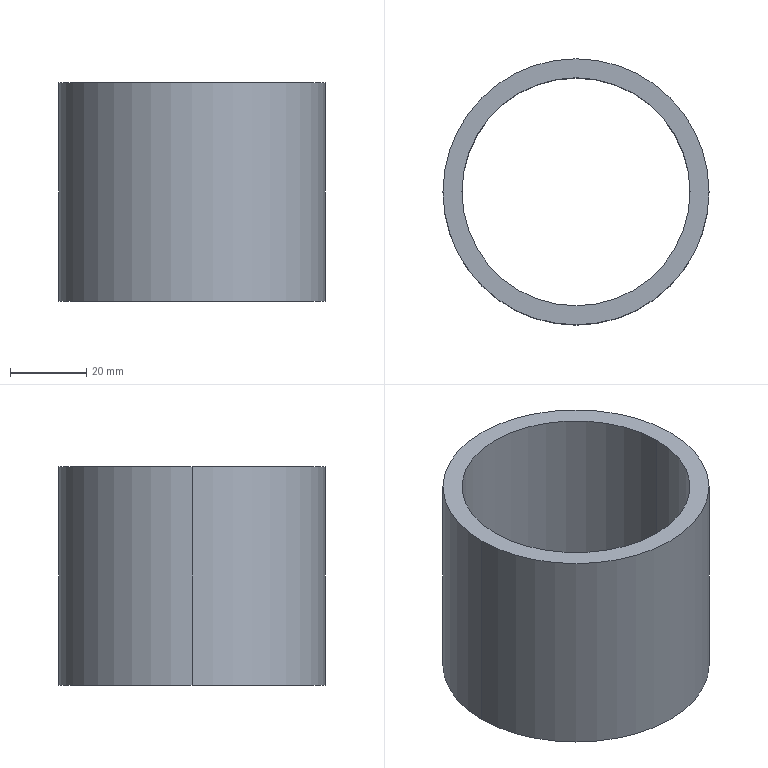Part | STEP file | 05-Spacer 2 | 1 solid | 6 faces | box 70 x 70 x 57.5 mm | volume 58709 mm3 | cylinder 4 | plane 2 | commonest cylinder face diameters 60 x2 70 x2
STEP:
#1=CARTESIAN_POINT('',(0.,0.,0.));
#2=DIRECTION('',(0.,0.,1.));
#3=DIRECTION('',(1.,0.,0.));
#4=AXIS2_PLACEMENT_3D('',#1,#2,#3);
#5=CARTESIAN_POINT('',(-30.,0.,57.5));
#6=VERTEX_POINT('',#5);
#7=CARTESIAN_POINT('',(-30.,0.,0.));
#8=VERTEX_POINT('',#7);
#9=CARTESIAN_POINT('',(-30.,0.,57.5));
#10=DIRECTION('',(0.,0.,-1.));
#11=VECTOR('',#10,1.);
#12=LINE('',#9,#11);
#13=CARTESIAN_POINT('',(0.,0.,57.5));
#14=DIRECTION('',(0.,0.,-1.));
#15=DIRECTION('',(-1.,0.,0.));
#16=AXIS2_PLACEMENT_3D('',#13,#14,#15);
#17=CYLINDRICAL_SURFACE('',#16,30.);
#18=CARTESIAN_POINT('',(6.283,0.));
#19=DIRECTION('',(0.,1.));
#20=VECTOR('',#19,1.);
#21=LINE('',#18,#20);
#22=(GEOMETRIC_REPRESENTATION_CONTEXT(2)PARAMETRIC_REPRESENTATION_CONTEXT()REPRESENTATION_CONTEXT('',''));
#23=DEFINITIONAL_REPRESENTATION('',(#21),#22);
#24=PCURVE('',#17,#23);
#25=CARTESIAN_POINT('',(0.,0.,57.5));
#26=DIRECTION('',(0.,0.,-1.));
#27=DIRECTION('',(-1.,0.,0.));
#28=AXIS2_PLACEMENT_3D('',#25,#26,#27);
#29=CYLINDRICAL_SURFACE('',#28,30.);
#30=CARTESIAN_POINT('',(0.,0.));
#31=DIRECTION('',(0.,1.));
#32=VECTOR('',#31,1.);
#33=LINE('',#30,#32);
#34=(GEOMETRIC_REPRESENTATION_CONTEXT(2)PARAMETRIC_REPRESENTATION_CONTEXT()REPRESENTATION_CONTEXT('',''));
#35=DEFINITIONAL_REPRESENTATION('',(#33),#34);
#36=PCURVE('',#29,#35);
#37=SURFACE_CURVE('',#12,(#24,#36),.PCURVE_S1.);
#38=EDGE_CURVE('',#6,#8,#37,.T.);
#39=ORIENTED_EDGE('',*,*,#38,.T.);
#40=CARTESIAN_POINT('',(30.,0.,0.));
#41=VERTEX_POINT('',#40);
#42=CARTESIAN_POINT('',(0.,0.,0.));
#43=DIRECTION('',(0.,0.,1.));
#44=DIRECTION('',(1.,0.,0.));
#45=AXIS2_PLACEMENT_3D('',#42,#43,#44);
#46=CIRCLE('',#45,30.);
#47=CARTESIAN_POINT('',(9.425,57.5));
#48=DIRECTION('',(-1.,0.));
#49=VECTOR('',#48,1.);
#50=LINE('',#47,#49);
#51=(GEOMETRIC_REPRESENTATION_CONTEXT(2)PARAMETRIC_REPRESENTATION_CONTEXT()REPRESENTATION_CONTEXT('',''));
#52=DEFINITIONAL_REPRESENTATION('',(#50),#51);
#53=PCURVE('',#17,#52);
#54=CARTESIAN_POINT('',(0.,0.,0.));
#55=DIRECTION('',(0.,0.,1.));
#56=DIRECTION('',(1.,0.,0.));
#57=AXIS2_PLACEMENT_3D('',#54,#55,#56);
#58=PLANE('',#57);
#59=CARTESIAN_POINT('',(0.,0.));
#60=DIRECTION('',(1.,0.));
#61=AXIS2_PLACEMENT_2D('',#59,#60);
#62=CIRCLE('',#61,30.);
#63=(GEOMETRIC_REPRESENTATION_CONTEXT(2)PARAMETRIC_REPRESENTATION_CONTEXT()REPRESENTATION_CONTEXT('',''));
#64=DEFINITIONAL_REPRESENTATION('',(#62),#63);
#65=PCURVE('',#58,#64);
#66=SURFACE_CURVE('',#46,(#53,#65),.PCURVE_S1.);
#67=EDGE_CURVE('',#8,#41,#66,.T.);
#68=ORIENTED_EDGE('',*,*,#67,.T.);
#69=CARTESIAN_POINT('',(30.,0.,57.5));
#70=VERTEX_POINT('',#69);
#71=CARTESIAN_POINT('',(30.,0.,57.5));
#72=DIRECTION('',(0.,0.,-1.));
#73=VECTOR('',#72,1.);
#74=LINE('',#71,#73);
#75=CARTESIAN_POINT('',(3.142,0.));
#76=DIRECTION('',(0.,1.));
#77=VECTOR('',#76,1.);
#78=LINE('',#75,#77);
#79=(GEOMETRIC_REPRESENTATION_CONTEXT(2)PARAMETRIC_REPRESENTATION_CONTEXT()REPRESENTATION_CONTEXT('',''));
#80=DEFINITIONAL_REPRESENTATION('',(#78),#79);
#81=PCURVE('',#17,#80);
#82=CARTESIAN_POINT('',(3.142,0.));
#83=DIRECTION('',(0.,1.));
#84=VECTOR('',#83,1.);
#85=LINE('',#82,#84);
#86=(GEOMETRIC_REPRESENTATION_CONTEXT(2)PARAMETRIC_REPRESENTATION_CONTEXT()REPRESENTATION_CONTEXT('',''));
#87=DEFINITIONAL_REPRESENTATION('',(#85),#86);
#88=PCURVE('',#29,#87);
#89=SURFACE_CURVE('',#74,(#81,#88),.PCURVE_S1.);
#90=EDGE_CURVE('',#70,#41,#89,.T.);
#91=ORIENTED_EDGE('',*,*,#90,.F.);
#92=CARTESIAN_POINT('',(0.,0.,57.5));
#93=DIRECTION('',(0.,0.,1.));
#94=DIRECTION('',(1.,0.,0.));
#95=AXIS2_PLACEMENT_3D('',#92,#93,#94);
#96=CIRCLE('',#95,30.);
#97=CARTESIAN_POINT('',(9.425,0.));
#98=DIRECTION('',(-1.,0.));
#99=VECTOR('',#98,1.);
#100=LINE('',#97,#99);
#101=(GEOMETRIC_REPRESENTATION_CONTEXT(2)PARAMETRIC_REPRESENTATION_CONTEXT()REPRESENTATION_CONTEXT('',''));
#102=DEFINITIONAL_REPRESENTATION('',(#100),#101);
#103=PCURVE('',#17,#102);
#104=CARTESIAN_POINT('',(0.,0.,57.5));
#105=DIRECTION('',(0.,0.,1.));
#106=DIRECTION('',(1.,0.,0.));
#107=AXIS2_PLACEMENT_3D('',#104,#105,#106);
#108=PLANE('',#107);
#109=CARTESIAN_POINT('',(0.,0.));
#110=DIRECTION('',(1.,0.));
#111=AXIS2_PLACEMENT_2D('',#109,#110);
#112=CIRCLE('',#111,30.);
#113=(GEOMETRIC_REPRESENTATION_CONTEXT(2)PARAMETRIC_REPRESENTATION_CONTEXT()REPRESENTATION_CONTEXT('',''));
#114=DEFINITIONAL_REPRESENTATION('',(#112),#113);
#115=PCURVE('',#108,#114);
#116=SURFACE_CURVE('',#96,(#103,#115),.PCURVE_S1.);
#117=EDGE_CURVE('',#6,#70,#116,.T.);
#118=ORIENTED_EDGE('',*,*,#117,.F.);
#119=EDGE_LOOP('',(#39,#68,#91,#118));
#120=FACE_BOUND('',#119,.F.);
#121=ADVANCED_FACE('',(#120),#17,.F.);
#122=CARTESIAN_POINT('',(35.,0.,57.5));
#123=VERTEX_POINT('',#122);
#124=CARTESIAN_POINT('',(-35.,0.,57.5));
#125=VERTEX_POINT('',#124);
#126=CARTESIAN_POINT('',(0.,0.,57.5));
#127=DIRECTION('',(0.,0.,1.));
#128=DIRECTION('',(1.,0.,0.));
#129=AXIS2_PLACEMENT_3D('',#126,#127,#128);
#130=CIRCLE('',#129,35.);
#131=CARTESIAN_POINT('',(0.,0.,57.5));
#132=DIRECTION('',(0.,0.,-1.));
#133=DIRECTION('',(-1.,0.,0.));
#134=AXIS2_PLACEMENT_3D('',#131,#132,#133);
#135=CYLINDRICAL_SURFACE('',#134,35.);
#136=CARTESIAN_POINT('',(3.142,0.));
#137=DIRECTION('',(-1.,0.));
#138=VECTOR('',#137,1.);
#139=LINE('',#136,#138);
#140=(GEOMETRIC_REPRESENTATION_CONTEXT(2)PARAMETRIC_REPRESENTATION_CONTEXT()REPRESENTATION_CONTEXT('',''));
#141=DEFINITIONAL_REPRESENTATION('',(#139),#140);
#142=PCURVE('',#135,#141);
#143=CARTESIAN_POINT('',(0.,0.));
#144=DIRECTION('',(1.,0.));
#145=AXIS2_PLACEMENT_2D('',#143,#144);
#146=CIRCLE('',#145,35.);
#147=(GEOMETRIC_REPRESENTATION_CONTEXT(2)PARAMETRIC_REPRESENTATION_CONTEXT()REPRESENTATION_CONTEXT('',''));
#148=DEFINITIONAL_REPRESENTATION('',(#146),#147);
#149=PCURVE('',#108,#148);
#150=SURFACE_CURVE('',#130,(#142,#149),.PCURVE_S1.);
#151=EDGE_CURVE('',#123,#125,#150,.T.);
#152=ORIENTED_EDGE('',*,*,#151,.F.);
#153=CARTESIAN_POINT('',(35.,0.,0.));
#154=VERTEX_POINT('',#153);
#155=CARTESIAN_POINT('',(35.,0.,57.5));
#156=DIRECTION('',(0.,0.,-1.));
#157=VECTOR('',#156,1.);
#158=LINE('',#155,#157);
#159=CARTESIAN_POINT('',(3.142,0.));
#160=DIRECTION('',(0.,1.));
#161=VECTOR('',#160,1.);
#162=LINE('',#159,#161);
#163=(GEOMETRIC_REPRESENTATION_CONTEXT(2)PARAMETRIC_REPRESENTATION_CONTEXT()REPRESENTATION_CONTEXT('',''));
#164=DEFINITIONAL_REPRESENTATION('',(#162),#163);
#165=PCURVE('',#135,#164);
#166=CARTESIAN_POINT('',(0.,0.,57.5));
#167=DIRECTION('',(0.,0.,-1.));
#168=DIRECTION('',(-1.,0.,0.));
#169=AXIS2_PLACEMENT_3D('',#166,#167,#168);
#170=CYLINDRICAL_SURFACE('',#169,35.);
#171=CARTESIAN_POINT('',(3.142,0.));
#172=DIRECTION('',(0.,1.));
#173=VECTOR('',#172,1.);
#174=LINE('',#171,#173);
#175=(GEOMETRIC_REPRESENTATION_CONTEXT(2)PARAMETRIC_REPRESENTATION_CONTEXT()REPRESENTATION_CONTEXT('',''));
#176=DEFINITIONAL_REPRESENTATION('',(#174),#175);
#177=PCURVE('',#170,#176);
#178=SURFACE_CURVE('',#158,(#165,#177),.PCURVE_S1.);
#179=EDGE_CURVE('',#123,#154,#178,.T.);
#180=ORIENTED_EDGE('',*,*,#179,.T.);
#181=CARTESIAN_POINT('',(-35.,0.,0.));
#182=VERTEX_POINT('',#181);
#183=CARTESIAN_POINT('',(0.,0.,0.));
#184=DIRECTION('',(0.,0.,1.));
#185=DIRECTION('',(1.,0.,0.));
#186=AXIS2_PLACEMENT_3D('',#183,#184,#185);
#187=CIRCLE('',#186,35.);
#188=CARTESIAN_POINT('',(3.142,57.5));
#189=DIRECTION('',(-1.,0.));
#190=VECTOR('',#189,1.);
#191=LINE('',#188,#190);
#192=(GEOMETRIC_REPRESENTATION_CONTEXT(2)PARAMETRIC_REPRESENTATION_CONTEXT()REPRESENTATION_CONTEXT('',''));
#193=DEFINITIONAL_REPRESENTATION('',(#191),#192);
#194=PCURVE('',#135,#193);
#195=CARTESIAN_POINT('',(0.,0.));
#196=DIRECTION('',(1.,0.));
#197=AXIS2_PLACEMENT_2D('',#195,#196);
#198=CIRCLE('',#197,35.);
#199=(GEOMETRIC_REPRESENTATION_CONTEXT(2)PARAMETRIC_REPRESENTATION_CONTEXT()REPRESENTATION_CONTEXT('',''));
#200=DEFINITIONAL_REPRESENTATION('',(#198),#199);
#201=PCURVE('',#58,#200);
#202=SURFACE_CURVE('',#187,(#194,#201),.PCURVE_S1.);
#203=EDGE_CURVE('',#154,#182,#202,.T.);
#204=ORIENTED_EDGE('',*,*,#203,.T.);
#205=CARTESIAN_POINT('',(-35.,0.,57.5));
#206=DIRECTION('',(0.,0.,-1.));
#207=VECTOR('',#206,1.);
#208=LINE('',#205,#207);
#209=CARTESIAN_POINT('',(0.,0.));
#210=DIRECTION('',(0.,1.));
#211=VECTOR('',#210,1.);
#212=LINE('',#209,#211);
#213=(GEOMETRIC_REPRESENTATION_CONTEXT(2)PARAMETRIC_REPRESENTATION_CONTEXT()REPRESENTATION_CONTEXT('',''));
#214=DEFINITIONAL_REPRESENTATION('',(#212),#213);
#215=PCURVE('',#135,#214);
#216=CARTESIAN_POINT('',(6.283,0.));
#217=DIRECTION('',(0.,1.));
#218=VECTOR('',#217,1.);
#219=LINE('',#216,#218);
#220=(GEOMETRIC_REPRESENTATION_CONTEXT(2)PARAMETRIC_REPRESENTATION_CONTEXT()REPRESENTATION_CONTEXT('',''));
#221=DEFINITIONAL_REPRESENTATION('',(#219),#220);
#222=PCURVE('',#170,#221);
#223=SURFACE_CURVE('',#208,(#215,#222),.PCURVE_S1.);
#224=EDGE_CURVE('',#125,#182,#223,.T.);
#225=ORIENTED_EDGE('',*,*,#224,.F.);
#226=EDGE_LOOP('',(#152,#180,#204,#225));
#227=FACE_BOUND('',#226,.T.);
#228=ADVANCED_FACE('',(#227),#135,.T.);
#229=CARTESIAN_POINT('',(0.,0.,57.5));
#230=DIRECTION('',(0.,0.,1.));
#231=DIRECTION('',(1.,0.,0.));
#232=AXIS2_PLACEMENT_3D('',#229,#230,#231);
#233=CIRCLE('',#232,35.);
#234=CARTESIAN_POINT('',(0.,0.));
#235=DIRECTION('',(1.,0.));
#236=AXIS2_PLACEMENT_2D('',#234,#235);
#237=CIRCLE('',#236,35.);
#238=(GEOMETRIC_REPRESENTATION_CONTEXT(2)PARAMETRIC_REPRESENTATION_CONTEXT()REPRESENTATION_CONTEXT('',''));
#239=DEFINITIONAL_REPRESENTATION('',(#237),#238);
#240=PCURVE('',#108,#239);
#241=CARTESIAN_POINT('',(9.425,0.));
#242=DIRECTION('',(-1.,0.));
#243=VECTOR('',#242,1.);
#244=LINE('',#241,#243);
#245=(GEOMETRIC_REPRESENTATION_CONTEXT(2)PARAMETRIC_REPRESENTATION_CONTEXT()REPRESENTATION_CONTEXT('',''));
#246=DEFINITIONAL_REPRESENTATION('',(#244),#245);
#247=PCURVE('',#170,#246);
#248=SURFACE_CURVE('',#233,(#240,#247),.PCURVE_S1.);
#249=EDGE_CURVE('',#125,#123,#248,.T.);
#250=ORIENTED_EDGE('',*,*,#249,.T.);
#251=ORIENTED_EDGE('',*,*,#151,.T.);
#252=EDGE_LOOP('',(#250,#251));
#253=FACE_BOUND('',#252,.T.);
#254=ORIENTED_EDGE('',*,*,#117,.F.);
#255=CARTESIAN_POINT('',(0.,0.,57.5));
#256=DIRECTION('',(0.,0.,1.));
#257=DIRECTION('',(1.,0.,0.));
#258=AXIS2_PLACEMENT_3D('',#255,#256,#257);
#259=CIRCLE('',#258,30.);
#260=CARTESIAN_POINT('',(0.,0.));
#261=DIRECTION('',(1.,0.));
#262=AXIS2_PLACEMENT_2D('',#260,#261);
#263=CIRCLE('',#262,30.);
#264=(GEOMETRIC_REPRESENTATION_CONTEXT(2)PARAMETRIC_REPRESENTATION_CONTEXT()REPRESENTATION_CONTEXT('',''));
#265=DEFINITIONAL_REPRESENTATION('',(#263),#264);
#266=PCURVE('',#108,#265);
#267=CARTESIAN_POINT('',(3.142,0.));
#268=DIRECTION('',(-1.,0.));
#269=VECTOR('',#268,1.);
#270=LINE('',#267,#269);
#271=(GEOMETRIC_REPRESENTATION_CONTEXT(2)PARAMETRIC_REPRESENTATION_CONTEXT()REPRESENTATION_CONTEXT('',''));
#272=DEFINITIONAL_REPRESENTATION('',(#270),#271);
#273=PCURVE('',#29,#272);
#274=SURFACE_CURVE('',#259,(#266,#273),.PCURVE_S1.);
#275=EDGE_CURVE('',#70,#6,#274,.T.);
#276=ORIENTED_EDGE('',*,*,#275,.F.);
#277=EDGE_LOOP('',(#254,#276));
#278=FACE_BOUND('',#277,.T.);
#279=ADVANCED_FACE('',(#253,#278),#108,.T.);
#280=CARTESIAN_POINT('',(0.,0.,0.));
#281=DIRECTION('',(0.,0.,1.));
#282=DIRECTION('',(1.,0.,0.));
#283=AXIS2_PLACEMENT_3D('',#280,#281,#282);
#284=CIRCLE('',#283,35.);
#285=CARTESIAN_POINT('',(0.,0.));
#286=DIRECTION('',(1.,0.));
#287=AXIS2_PLACEMENT_2D('',#285,#286);
#288=CIRCLE('',#287,35.);
#289=(GEOMETRIC_REPRESENTATION_CONTEXT(2)PARAMETRIC_REPRESENTATION_CONTEXT()REPRESENTATION_CONTEXT('',''));
#290=DEFINITIONAL_REPRESENTATION('',(#288),#289);
#291=PCURVE('',#58,#290);
#292=CARTESIAN_POINT('',(9.425,57.5));
#293=DIRECTION('',(-1.,0.));
#294=VECTOR('',#293,1.);
#295=LINE('',#292,#294);
#296=(GEOMETRIC_REPRESENTATION_CONTEXT(2)PARAMETRIC_REPRESENTATION_CONTEXT()REPRESENTATION_CONTEXT('',''));
#297=DEFINITIONAL_REPRESENTATION('',(#295),#296);
#298=PCURVE('',#170,#297);
#299=SURFACE_CURVE('',#284,(#291,#298),.PCURVE_S1.);
#300=EDGE_CURVE('',#182,#154,#299,.T.);
#301=ORIENTED_EDGE('',*,*,#300,.F.);
#302=ORIENTED_EDGE('',*,*,#203,.F.);
#303=EDGE_LOOP('',(#301,#302));
#304=FACE_BOUND('',#303,.T.);
#305=ORIENTED_EDGE('',*,*,#67,.T.);
#306=CARTESIAN_POINT('',(0.,0.,0.));
#307=DIRECTION('',(0.,0.,1.));
#308=DIRECTION('',(1.,0.,0.));
#309=AXIS2_PLACEMENT_3D('',#306,#307,#308);
#310=CIRCLE('',#309,30.);
#311=CARTESIAN_POINT('',(0.,0.));
#312=DIRECTION('',(1.,0.));
#313=AXIS2_PLACEMENT_2D('',#311,#312);
#314=CIRCLE('',#313,30.);
#315=(GEOMETRIC_REPRESENTATION_CONTEXT(2)PARAMETRIC_REPRESENTATION_CONTEXT()REPRESENTATION_CONTEXT('',''));
#316=DEFINITIONAL_REPRESENTATION('',(#314),#315);
#317=PCURVE('',#58,#316);
#318=CARTESIAN_POINT('',(3.142,57.5));
#319=DIRECTION('',(-1.,0.));
#320=VECTOR('',#319,1.);
#321=LINE('',#318,#320);
#322=(GEOMETRIC_REPRESENTATION_CONTEXT(2)PARAMETRIC_REPRESENTATION_CONTEXT()REPRESENTATION_CONTEXT('',''));
#323=DEFINITIONAL_REPRESENTATION('',(#321),#322);
#324=PCURVE('',#29,#323);
#325=SURFACE_CURVE('',#310,(#317,#324),.PCURVE_S1.);
#326=EDGE_CURVE('',#41,#8,#325,.T.);
#327=ORIENTED_EDGE('',*,*,#326,.T.);
#328=EDGE_LOOP('',(#305,#327));
#329=FACE_BOUND('',#328,.T.);
#330=ADVANCED_FACE('',(#304,#329),#58,.F.);
#331=ORIENTED_EDGE('',*,*,#179,.F.);
#332=ORIENTED_EDGE('',*,*,#249,.F.);
#333=ORIENTED_EDGE('',*,*,#224,.T.);
#334=ORIENTED_EDGE('',*,*,#300,.T.);
#335=EDGE_LOOP('',(#331,#332,#333,#334));
#336=FACE_BOUND('',#335,.T.);
#337=ADVANCED_FACE('',(#336),#170,.T.);
#338=ORIENTED_EDGE('',*,*,#326,.T.);
#339=ORIENTED_EDGE('',*,*,#38,.F.);
#340=ORIENTED_EDGE('',*,*,#275,.F.);
#341=ORIENTED_EDGE('',*,*,#90,.T.);
#342=EDGE_LOOP('',(#338,#339,#340,#341));
#343=FACE_BOUND('',#342,.F.);
#344=ADVANCED_FACE('',(#343),#29,.F.);
#345=CLOSED_SHELL('',(#121,#228,#279,#330,#337,#344));
#346=MANIFOLD_SOLID_BREP('',#345);
#347=(LENGTH_UNIT()NAMED_UNIT(*)SI_UNIT(.MILLI.,.METRE.));
#348=UNCERTAINTY_MEASURE_WITH_UNIT(LENGTH_MEASURE(0.0000001),#347,'','');
#349=(NAMED_UNIT(*)PLANE_ANGLE_UNIT()SI_UNIT($,.RADIAN.));
#350=(NAMED_UNIT(*)SI_UNIT($,.STERADIAN.)SOLID_ANGLE_UNIT());
#351=(GEOMETRIC_REPRESENTATION_CONTEXT(3)GLOBAL_UNCERTAINTY_ASSIGNED_CONTEXT((#348))GLOBAL_UNIT_ASSIGNED_CONTEXT((#347,#349,#350))REPRESENTATION_CONTEXT('',''));
#352=ADVANCED_BREP_SHAPE_REPRESENTATION('',(#4,#346),#351);